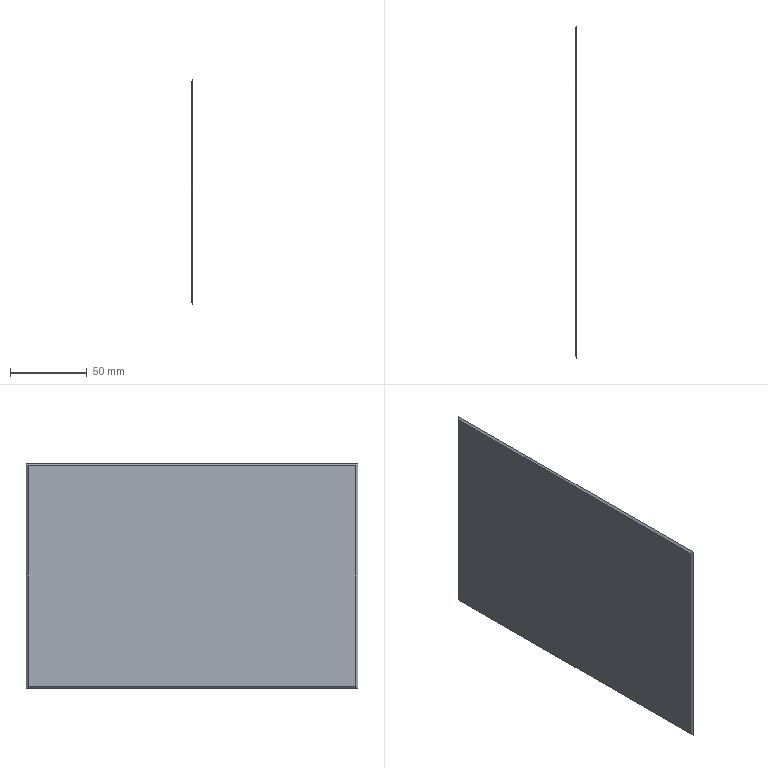Part | NX | 1 solid | 6 faces | box 1.2 x 216.4 x 146.4 mm | volume 37497 mm3 | plane 6
STEP:
#1=CARTESIAN_POINT('',(-120.,-107.,-72.));
#2=VERTEX_POINT('',#1);
#3=CARTESIAN_POINT('',(-120.,107.,-72.));
#4=VERTEX_POINT('',#3);
#5=CARTESIAN_POINT('',(-120.,0.,-72.));
#6=DIRECTION('',(0.,1.,0.));
#7=VECTOR('',#6,1000.);
#8=LINE('',#5,#7);
#9=EDGE_CURVE('',#2,#4,#8,.T.);
#10=ORIENTED_EDGE('',*,*,#9,.F.);
#11=CARTESIAN_POINT('',(-120.,-107.,72.));
#12=VERTEX_POINT('',#11);
#13=CARTESIAN_POINT('',(-120.,-107.,0.));
#14=DIRECTION('',(0.,0.,-1.));
#15=VECTOR('',#14,1000.);
#16=LINE('',#13,#15);
#17=EDGE_CURVE('',#12,#2,#16,.T.);
#18=ORIENTED_EDGE('',*,*,#17,.F.);
#19=CARTESIAN_POINT('',(-120.,107.,72.));
#20=VERTEX_POINT('',#19);
#21=CARTESIAN_POINT('',(-120.,0.,72.));
#22=DIRECTION('',(0.,1.,0.));
#23=VECTOR('',#22,1000.);
#24=LINE('',#21,#23);
#25=EDGE_CURVE('',#12,#20,#24,.T.);
#26=ORIENTED_EDGE('',*,*,#25,.T.);
#27=CARTESIAN_POINT('',(-120.,107.,0.));
#28=DIRECTION('',(0.,0.,-1.));
#29=VECTOR('',#28,1000.);
#30=LINE('',#27,#29);
#31=EDGE_CURVE('',#20,#4,#30,.T.);
#32=ORIENTED_EDGE('',*,*,#31,.T.);
#33=EDGE_LOOP('',(#10,#18,#26,#32));
#34=FACE_BOUND('',#33,.T.);
#35=CARTESIAN_POINT('',(-120.,110.,-75.));
#36=DIRECTION('',(-1.,0.,0.));
#37=DIRECTION('',(0.,0.,1.));
#38=AXIS2_PLACEMENT_3D('',#35,#36,#37);
#39=PLANE('',#38);
#40=ADVANCED_FACE('',(#34),#39,.T.);
#41=CARTESIAN_POINT('',(-118.8,108.2,-73.2));
#42=VERTEX_POINT('',#41);
#43=CARTESIAN_POINT('',(-118.8,-108.2,-73.2));
#44=VERTEX_POINT('',#43);
#45=CARTESIAN_POINT('',(-118.8,0.,-73.2));
#46=DIRECTION('',(0.,-1.,0.));
#47=VECTOR('',#46,1000.);
#48=LINE('',#45,#47);
#49=EDGE_CURVE('',#42,#44,#48,.T.);
#50=ORIENTED_EDGE('',*,*,#49,.T.);
#51=CARTESIAN_POINT('',(-192.,-35.,0.));
#52=DIRECTION('',(-0.5774,0.5774,0.5774));
#53=VECTOR('',#52,1000.);
#54=LINE('',#51,#53);
#55=EDGE_CURVE('',#44,#2,#54,.T.);
#56=ORIENTED_EDGE('',*,*,#55,.T.);
#57=ORIENTED_EDGE('',*,*,#9,.T.);
#58=CARTESIAN_POINT('',(-192.,35.,0.));
#59=DIRECTION('',(-0.5774,-0.5774,0.5774));
#60=VECTOR('',#59,1000.);
#61=LINE('',#58,#60);
#62=EDGE_CURVE('',#42,#4,#61,.T.);
#63=ORIENTED_EDGE('',*,*,#62,.F.);
#64=EDGE_LOOP('',(#50,#56,#57,#63));
#65=FACE_BOUND('',#64,.T.);
#66=CARTESIAN_POINT('',(-118.5,0.,-73.5));
#67=DIRECTION('',(-0.7071,0.,-0.7071));
#68=DIRECTION('',(-0.7071,0.,0.7071));
#69=AXIS2_PLACEMENT_3D('',#66,#67,#68);
#70=PLANE('',#69);
#71=ADVANCED_FACE('',(#65),#70,.T.);
#72=CARTESIAN_POINT('',(-118.8,108.2,73.2));
#73=VERTEX_POINT('',#72);
#74=CARTESIAN_POINT('',(-118.8,108.2,0.));
#75=DIRECTION('',(0.,0.,1.));
#76=VECTOR('',#75,1000.);
#77=LINE('',#74,#76);
#78=EDGE_CURVE('',#42,#73,#77,.T.);
#79=ORIENTED_EDGE('',*,*,#78,.F.);
#80=ORIENTED_EDGE('',*,*,#62,.T.);
#81=ORIENTED_EDGE('',*,*,#31,.F.);
#82=CARTESIAN_POINT('',(-192.,35.,0.));
#83=DIRECTION('',(-0.5774,-0.5774,-0.5774));
#84=VECTOR('',#83,1000.);
#85=LINE('',#82,#84);
#86=EDGE_CURVE('',#73,#20,#85,.T.);
#87=ORIENTED_EDGE('',*,*,#86,.F.);
#88=EDGE_LOOP('',(#79,#80,#81,#87));
#89=FACE_BOUND('',#88,.T.);
#90=CARTESIAN_POINT('',(-118.5,108.5,0.));
#91=DIRECTION('',(0.7071,-0.7071,0.));
#92=DIRECTION('',(0.,0.,-1.));
#93=AXIS2_PLACEMENT_3D('',#90,#91,#92);
#94=PLANE('',#93);
#95=ADVANCED_FACE('',(#89),#94,.F.);
#96=CARTESIAN_POINT('',(-118.8,-108.2,73.2));
#97=VERTEX_POINT('',#96);
#98=CARTESIAN_POINT('',(-118.8,-108.2,0.));
#99=DIRECTION('',(0.,0.,1.));
#100=VECTOR('',#99,1000.);
#101=LINE('',#98,#100);
#102=EDGE_CURVE('',#44,#97,#101,.T.);
#103=ORIENTED_EDGE('',*,*,#102,.F.);
#104=ORIENTED_EDGE('',*,*,#49,.F.);
#105=ORIENTED_EDGE('',*,*,#78,.T.);
#106=CARTESIAN_POINT('',(-118.8,0.,73.2));
#107=DIRECTION('',(0.,-1.,0.));
#108=VECTOR('',#107,1000.);
#109=LINE('',#106,#108);
#110=EDGE_CURVE('',#73,#97,#109,.T.);
#111=ORIENTED_EDGE('',*,*,#110,.T.);
#112=EDGE_LOOP('',(#103,#104,#105,#111));
#113=FACE_BOUND('',#112,.T.);
#114=CARTESIAN_POINT('',(-118.8,110.,-75.));
#115=DIRECTION('',(-1.,0.,0.));
#116=DIRECTION('',(0.,0.,1.));
#117=AXIS2_PLACEMENT_3D('',#114,#115,#116);
#118=PLANE('',#117);
#119=ADVANCED_FACE('',(#113),#118,.F.);
#120=ORIENTED_EDGE('',*,*,#110,.F.);
#121=ORIENTED_EDGE('',*,*,#86,.T.);
#122=ORIENTED_EDGE('',*,*,#25,.F.);
#123=CARTESIAN_POINT('',(-192.,-35.,0.));
#124=DIRECTION('',(-0.5774,0.5774,-0.5774));
#125=VECTOR('',#124,1000.);
#126=LINE('',#123,#125);
#127=EDGE_CURVE('',#97,#12,#126,.T.);
#128=ORIENTED_EDGE('',*,*,#127,.F.);
#129=EDGE_LOOP('',(#120,#121,#122,#128));
#130=FACE_BOUND('',#129,.T.);
#131=CARTESIAN_POINT('',(-118.5,0.,73.5));
#132=DIRECTION('',(0.7071,0.,-0.7071));
#133=DIRECTION('',(0.,-1.,0.));
#134=AXIS2_PLACEMENT_3D('',#131,#132,#133);
#135=PLANE('',#134);
#136=ADVANCED_FACE('',(#130),#135,.F.);
#137=ORIENTED_EDGE('',*,*,#102,.T.);
#138=ORIENTED_EDGE('',*,*,#127,.T.);
#139=ORIENTED_EDGE('',*,*,#17,.T.);
#140=ORIENTED_EDGE('',*,*,#55,.F.);
#141=EDGE_LOOP('',(#137,#138,#139,#140));
#142=FACE_BOUND('',#141,.T.);
#143=CARTESIAN_POINT('',(-118.5,-108.5,0.));
#144=DIRECTION('',(-0.7071,-0.7071,0.));
#145=DIRECTION('',(-0.7071,0.7071,0.));
#146=AXIS2_PLACEMENT_3D('',#143,#144,#145);
#147=PLANE('',#146);
#148=ADVANCED_FACE('',(#142),#147,.T.);
#149=CLOSED_SHELL('',(#40,#71,#95,#119,#136,#148));
#150=MANIFOLD_SOLID_BREP('',#149);
#151=(LENGTH_UNIT()NAMED_UNIT(*)SI_UNIT(.MILLI.,.METRE.));
#152=UNCERTAINTY_MEASURE_WITH_UNIT(LENGTH_MEASURE(0.00001),#151,'','');
#153=(NAMED_UNIT(*)PLANE_ANGLE_UNIT()SI_UNIT($,.RADIAN.));
#154=(NAMED_UNIT(*)SI_UNIT($,.STERADIAN.)SOLID_ANGLE_UNIT());
#155=(GEOMETRIC_REPRESENTATION_CONTEXT(3)GLOBAL_UNCERTAINTY_ASSIGNED_CONTEXT((#152))GLOBAL_UNIT_ASSIGNED_CONTEXT((#151,#153,#154))REPRESENTATION_CONTEXT('',''));
#156=ADVANCED_BREP_SHAPE_REPRESENTATION('',(#150),#155);